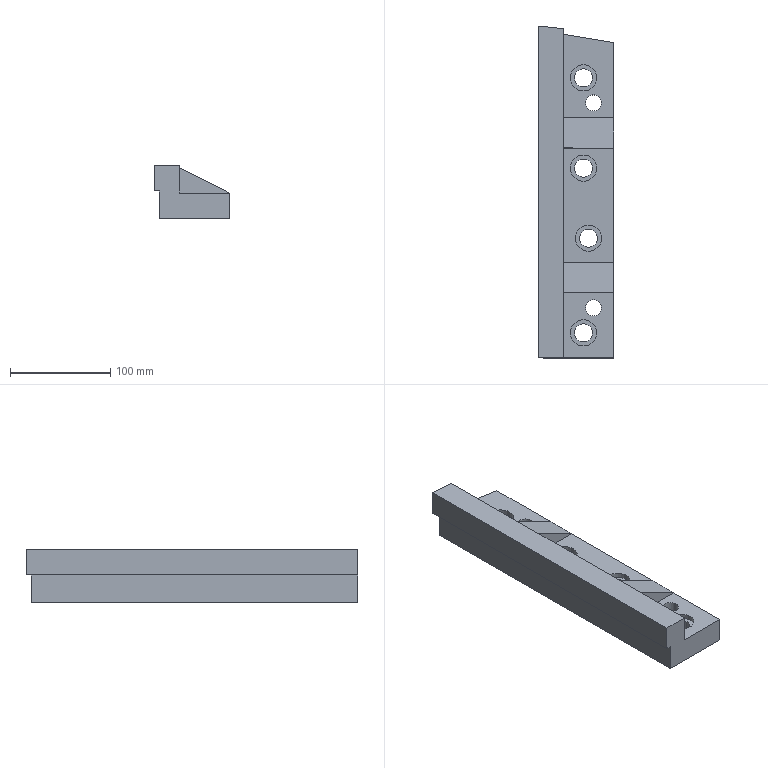Part | NX | features solid 2 | 1 solid | 33 faces | box 75 x 331.183 x 52 mm | volume 776457 mm3 | plane 21 | cylinder 10 | spline 2 | commonest cylinder face diameters 18 x4 26 x4 16 x2
STEP:
#1=CARTESIAN_POINT('',(-267.,-375.538,-30.));
#2=VERTEX_POINT('',#1);
#3=CARTESIAN_POINT('',(-280.,-375.538,-30.));
#4=DIRECTION('',(0.,0.,-1.));
#5=DIRECTION('',(1.,0.,0.));
#6=AXIS2_PLACEMENT_3D('',#3,#4,#5);
#7=CIRCLE('',#6,13.);
#8=EDGE_CURVE('',#2,#2,#7,.T.);
#9=ORIENTED_EDGE('',*,*,#8,.T.);
#10=EDGE_LOOP('',(#9));
#11=FACE_BOUND('',#10,.T.);
#12=CARTESIAN_POINT('',(-262.,-445.538,-30.));
#13=VERTEX_POINT('',#12);
#14=CARTESIAN_POINT('',(-275.,-445.538,-30.));
#15=DIRECTION('',(0.,0.,-1.));
#16=DIRECTION('',(1.,0.,0.));
#17=AXIS2_PLACEMENT_3D('',#14,#15,#16);
#18=CIRCLE('',#17,13.);
#19=EDGE_CURVE('',#13,#13,#18,.T.);
#20=ORIENTED_EDGE('',*,*,#19,.T.);
#21=EDGE_LOOP('',(#20));
#22=FACE_BOUND('',#21,.T.);
#23=CARTESIAN_POINT('',(-250.,-470.,-30.));
#24=VERTEX_POINT('',#23);
#25=CARTESIAN_POINT('',(-250.,-355.538,-30.));
#26=VERTEX_POINT('',#25);
#27=CARTESIAN_POINT('',(-250.,-560.,-30.));
#28=DIRECTION('',(0.,1.,0.));
#29=VECTOR('',#28,1000.);
#30=LINE('',#27,#29);
#31=EDGE_CURVE('',#24,#26,#30,.T.);
#32=ORIENTED_EDGE('',*,*,#31,.T.);
#33=CARTESIAN_POINT('',(-300.,-355.538,-30.));
#34=VERTEX_POINT('',#33);
#35=CARTESIAN_POINT('',(-300.,-355.538,-30.));
#36=DIRECTION('',(1.,0.,0.));
#37=VECTOR('',#36,1000.);
#38=LINE('',#35,#37);
#39=EDGE_CURVE('',#34,#26,#38,.T.);
#40=ORIENTED_EDGE('',*,*,#39,.F.);
#41=CARTESIAN_POINT('',(-300.,-470.,-30.));
#42=VERTEX_POINT('',#41);
#43=CARTESIAN_POINT('',(-300.,-560.,-30.));
#44=DIRECTION('',(0.,1.,0.));
#45=VECTOR('',#44,1000.);
#46=LINE('',#43,#45);
#47=EDGE_CURVE('',#42,#34,#46,.T.);
#48=ORIENTED_EDGE('',*,*,#47,.F.);
#49=CARTESIAN_POINT('',(-300.,-470.,-30.));
#50=DIRECTION('',(1.,0.,0.));
#51=VECTOR('',#50,1000.);
#52=LINE('',#49,#51);
#53=EDGE_CURVE('',#42,#24,#52,.T.);
#54=ORIENTED_EDGE('',*,*,#53,.T.);
#55=EDGE_LOOP('',(#32,#40,#48,#54));
#56=FACE_BOUND('',#55,.T.);
#57=CARTESIAN_POINT('',(-272.356,-257.29,-30.));
#58=DIRECTION('',(0.,0.,-1.));
#59=DIRECTION('',(-1.,0.,0.));
#60=AXIS2_PLACEMENT_3D('',#57,#58,#59);
#61=PLANE('',#60);
#62=ADVANCED_FACE('',(#11,#22,#56),#61,.F.);
#63=CARTESIAN_POINT('',(-267.,-285.538,-30.));
#64=VERTEX_POINT('',#63);
#65=CARTESIAN_POINT('',(-280.,-285.538,-30.));
#66=DIRECTION('',(0.,0.,-1.));
#67=DIRECTION('',(1.,0.,0.));
#68=AXIS2_PLACEMENT_3D('',#65,#66,#67);
#69=CIRCLE('',#68,13.);
#70=EDGE_CURVE('',#64,#64,#69,.T.);
#71=ORIENTED_EDGE('',*,*,#70,.T.);
#72=EDGE_LOOP('',(#71));
#73=FACE_BOUND('',#72,.T.);
#74=CARTESIAN_POINT('',(-262.,-310.538,-30.));
#75=VERTEX_POINT('',#74);
#76=CARTESIAN_POINT('',(-270.,-310.538,-30.));
#77=DIRECTION('',(0.,0.,-1.));
#78=DIRECTION('',(1.,0.,0.));
#79=AXIS2_PLACEMENT_3D('',#76,#77,#78);
#80=CIRCLE('',#79,8.);
#81=EDGE_CURVE('',#75,#75,#80,.T.);
#82=ORIENTED_EDGE('',*,*,#81,.T.);
#83=EDGE_LOOP('',(#82));
#84=FACE_BOUND('',#83,.T.);
#85=CARTESIAN_POINT('',(-300.,-325.538,-30.));
#86=VERTEX_POINT('',#85);
#87=CARTESIAN_POINT('',(-300.,-241.994,-30.));
#88=VERTEX_POINT('',#87);
#89=CARTESIAN_POINT('',(-300.,-560.,-30.));
#90=DIRECTION('',(0.,1.,0.));
#91=VECTOR('',#90,1000.);
#92=LINE('',#89,#91);
#93=EDGE_CURVE('',#86,#88,#92,.T.);
#94=ORIENTED_EDGE('',*,*,#93,.F.);
#95=CARTESIAN_POINT('',(-250.,-325.538,-30.));
#96=VERTEX_POINT('',#95);
#97=CARTESIAN_POINT('',(-300.,-325.538,-30.));
#98=DIRECTION('',(1.,0.,0.));
#99=VECTOR('',#98,1000.);
#100=LINE('',#97,#99);
#101=EDGE_CURVE('',#86,#96,#100,.T.);
#102=ORIENTED_EDGE('',*,*,#101,.T.);
#103=CARTESIAN_POINT('',(-250.,-250.331,-30.));
#104=VERTEX_POINT('',#103);
#105=CARTESIAN_POINT('',(-250.,-560.,-30.));
#106=DIRECTION('',(0.,1.,0.));
#107=VECTOR('',#106,1000.);
#108=LINE('',#105,#107);
#109=EDGE_CURVE('',#96,#104,#108,.T.);
#110=ORIENTED_EDGE('',*,*,#109,.T.);
#111=CARTESIAN_POINT('',(-250.,-250.331,-30.));
#112=CARTESIAN_POINT('',(-266.667,-247.552,-30.));
#113=CARTESIAN_POINT('',(-283.328,-244.74,-30.));
#114=CARTESIAN_POINT('',(-300.,-241.994,-30.));
#115=B_SPLINE_CURVE_WITH_KNOTS('',3,(#111,#112,#113,#114),.UNSPECIFIED.,.F.,.F.,(4,4),(0.3212,0.3719),.UNSPECIFIED.);
#116=EDGE_CURVE('',#104,#88,#115,.T.);
#117=ORIENTED_EDGE('',*,*,#116,.T.);
#118=EDGE_LOOP('',(#94,#102,#110,#117));
#119=FACE_BOUND('',#118,.T.);
#120=CARTESIAN_POINT('',(-272.356,-257.29,-30.));
#121=DIRECTION('',(0.,0.,-1.));
#122=DIRECTION('',(-1.,0.,0.));
#123=AXIS2_PLACEMENT_3D('',#120,#121,#122);
#124=PLANE('',#123);
#125=ADVANCED_FACE('',(#73,#84,#119),#124,.F.);
#126=CARTESIAN_POINT('',(-250.,-565.,-30.));
#127=VERTEX_POINT('',#126);
#128=CARTESIAN_POINT('',(-250.,-500.,-30.));
#129=VERTEX_POINT('',#128);
#130=CARTESIAN_POINT('',(-250.,-560.,-30.));
#131=DIRECTION('',(0.,1.,0.));
#132=VECTOR('',#131,1000.);
#133=LINE('',#130,#132);
#134=EDGE_CURVE('',#127,#129,#133,.T.);
#135=ORIENTED_EDGE('',*,*,#134,.T.);
#136=CARTESIAN_POINT('',(-300.,-500.,-30.));
#137=VERTEX_POINT('',#136);
#138=CARTESIAN_POINT('',(-300.,-500.,-30.));
#139=DIRECTION('',(1.,0.,0.));
#140=VECTOR('',#139,1000.);
#141=LINE('',#138,#140);
#142=EDGE_CURVE('',#137,#129,#141,.T.);
#143=ORIENTED_EDGE('',*,*,#142,.F.);
#144=CARTESIAN_POINT('',(-300.,-565.,-30.));
#145=VERTEX_POINT('',#144);
#146=CARTESIAN_POINT('',(-300.,-560.,-30.));
#147=DIRECTION('',(0.,1.,0.));
#148=VECTOR('',#147,1000.);
#149=LINE('',#146,#148);
#150=EDGE_CURVE('',#145,#137,#149,.T.);
#151=ORIENTED_EDGE('',*,*,#150,.F.);
#152=CARTESIAN_POINT('',(-245.,-565.,-30.));
#153=DIRECTION('',(-1.,0.,0.));
#154=VECTOR('',#153,1000.);
#155=LINE('',#152,#154);
#156=EDGE_CURVE('',#127,#145,#155,.T.);
#157=ORIENTED_EDGE('',*,*,#156,.F.);
#158=EDGE_LOOP('',(#135,#143,#151,#157));
#159=FACE_BOUND('',#158,.T.);
#160=CARTESIAN_POINT('',(-262.,-515.,-30.));
#161=VERTEX_POINT('',#160);
#162=CARTESIAN_POINT('',(-270.,-515.,-30.));
#163=DIRECTION('',(0.,0.,1.));
#164=DIRECTION('',(1.,0.,0.));
#165=AXIS2_PLACEMENT_3D('',#162,#163,#164);
#166=CIRCLE('',#165,8.);
#167=EDGE_CURVE('',#161,#161,#166,.T.);
#168=ORIENTED_EDGE('',*,*,#167,.F.);
#169=EDGE_LOOP('',(#168));
#170=FACE_BOUND('',#169,.T.);
#171=CARTESIAN_POINT('',(-267.,-540.,-30.));
#172=VERTEX_POINT('',#171);
#173=CARTESIAN_POINT('',(-280.,-540.,-30.));
#174=DIRECTION('',(0.,0.,1.));
#175=DIRECTION('',(1.,0.,0.));
#176=AXIS2_PLACEMENT_3D('',#173,#174,#175);
#177=CIRCLE('',#176,13.);
#178=EDGE_CURVE('',#172,#172,#177,.T.);
#179=ORIENTED_EDGE('',*,*,#178,.F.);
#180=EDGE_LOOP('',(#179));
#181=FACE_BOUND('',#180,.T.);
#182=CARTESIAN_POINT('',(-272.356,-257.29,-30.));
#183=DIRECTION('',(0.,0.,-1.));
#184=DIRECTION('',(-1.,0.,0.));
#185=AXIS2_PLACEMENT_3D('',#182,#183,#184);
#186=PLANE('',#185);
#187=ADVANCED_FACE('',(#159,#170,#181),#186,.F.);
#188=CARTESIAN_POINT('',(-289.,-540.,-55.));
#189=VERTEX_POINT('',#188);
#190=CARTESIAN_POINT('',(-280.,-540.,-55.));
#191=DIRECTION('',(0.,0.,-1.));
#192=DIRECTION('',(-1.,0.,0.));
#193=AXIS2_PLACEMENT_3D('',#190,#191,#192);
#194=CIRCLE('',#193,9.);
#195=EDGE_CURVE('',#189,#189,#194,.T.);
#196=ORIENTED_EDGE('',*,*,#195,.T.);
#197=EDGE_LOOP('',(#196));
#198=FACE_BOUND('',#197,.T.);
#199=CARTESIAN_POINT('',(-271.,-540.,-35.));
#200=VERTEX_POINT('',#199);
#201=CARTESIAN_POINT('',(-280.,-540.,-35.));
#202=DIRECTION('',(0.,0.,1.));
#203=DIRECTION('',(1.,0.,0.));
#204=AXIS2_PLACEMENT_3D('',#201,#202,#203);
#205=CIRCLE('',#204,9.);
#206=EDGE_CURVE('',#200,#200,#205,.F.);
#207=ORIENTED_EDGE('',*,*,#206,.F.);
#208=EDGE_LOOP('',(#207));
#209=FACE_BOUND('',#208,.T.);
#210=CARTESIAN_POINT('',(-280.,-540.,-60.));
#211=DIRECTION('',(0.,0.,1.));
#212=DIRECTION('',(1.,0.,0.));
#213=AXIS2_PLACEMENT_3D('',#210,#211,#212);
#214=CYLINDRICAL_SURFACE('',#213,9.);
#215=ADVANCED_FACE('',(#198,#209),#214,.F.);
#216=ORIENTED_EDGE('',*,*,#195,.F.);
#217=EDGE_LOOP('',(#216));
#218=FACE_BOUND('',#217,.T.);
#219=CARTESIAN_POINT('',(-278.,-515.,-55.));
#220=VERTEX_POINT('',#219);
#221=CARTESIAN_POINT('',(-270.,-515.,-55.));
#222=DIRECTION('',(0.,0.,-1.));
#223=DIRECTION('',(-1.,0.,0.));
#224=AXIS2_PLACEMENT_3D('',#221,#222,#223);
#225=CIRCLE('',#224,8.);
#226=EDGE_CURVE('',#220,#220,#225,.T.);
#227=ORIENTED_EDGE('',*,*,#226,.F.);
#228=EDGE_LOOP('',(#227));
#229=FACE_BOUND('',#228,.T.);
#230=CARTESIAN_POINT('',(-289.,-375.538,-55.));
#231=VERTEX_POINT('',#230);
#232=CARTESIAN_POINT('',(-280.,-375.538,-55.));
#233=DIRECTION('',(0.,0.,-1.));
#234=DIRECTION('',(-1.,0.,0.));
#235=AXIS2_PLACEMENT_3D('',#232,#233,#234);
#236=CIRCLE('',#235,9.);
#237=EDGE_CURVE('',#231,#231,#236,.F.);
#238=ORIENTED_EDGE('',*,*,#237,.T.);
#239=EDGE_LOOP('',(#238));
#240=FACE_BOUND('',#239,.T.);
#241=CARTESIAN_POINT('',(-289.,-285.538,-55.));
#242=VERTEX_POINT('',#241);
#243=CARTESIAN_POINT('',(-280.,-285.538,-55.));
#244=DIRECTION('',(0.,0.,-1.));
#245=DIRECTION('',(-1.,0.,0.));
#246=AXIS2_PLACEMENT_3D('',#243,#244,#245);
#247=CIRCLE('',#246,9.);
#248=EDGE_CURVE('',#242,#242,#247,.F.);
#249=ORIENTED_EDGE('',*,*,#248,.T.);
#250=EDGE_LOOP('',(#249));
#251=FACE_BOUND('',#250,.T.);
#252=CARTESIAN_POINT('',(-250.,-250.331,-55.));
#253=VERTEX_POINT('',#252);
#254=CARTESIAN_POINT('',(-320.,-238.927,-55.));
#255=VERTEX_POINT('',#254);
#256=CARTESIAN_POINT('',(-250.,-250.331,-55.));
#257=CARTESIAN_POINT('',(-261.66,-248.387,-55.));
#258=CARTESIAN_POINT('',(-284.979,-244.502,-55.));
#259=CARTESIAN_POINT('',(-308.296,-240.6,-55.));
#260=CARTESIAN_POINT('',(-320.,-238.927,-55.));
#261=B_SPLINE_CURVE_WITH_KNOTS('',3,(#256,#257,#258,#259,#260),.UNSPECIFIED.,.F.,.F.,(4,1,4),(0.,0.03546,0.07092),.UNSPECIFIED.);
#262=EDGE_CURVE('',#253,#255,#261,.T.);
#263=ORIENTED_EDGE('',*,*,#262,.F.);
#264=CARTESIAN_POINT('',(-250.,-565.,-55.));
#265=VERTEX_POINT('',#264);
#266=CARTESIAN_POINT('',(-250.,-560.,-55.));
#267=DIRECTION('',(0.,1.,0.));
#268=VECTOR('',#267,1000.);
#269=LINE('',#266,#268);
#270=EDGE_CURVE('',#265,#253,#269,.T.);
#271=ORIENTED_EDGE('',*,*,#270,.F.);
#272=CARTESIAN_POINT('',(-320.,-565.,-55.));
#273=VERTEX_POINT('',#272);
#274=CARTESIAN_POINT('',(-245.,-565.,-55.));
#275=DIRECTION('',(-1.,0.,0.));
#276=VECTOR('',#275,1000.);
#277=LINE('',#274,#276);
#278=EDGE_CURVE('',#265,#273,#277,.T.);
#279=ORIENTED_EDGE('',*,*,#278,.T.);
#280=CARTESIAN_POINT('',(-320.,-257.29,-55.));
#281=DIRECTION('',(0.,1.,0.));
#282=VECTOR('',#281,1000.);
#283=LINE('',#280,#282);
#284=EDGE_CURVE('',#273,#255,#283,.T.);
#285=ORIENTED_EDGE('',*,*,#284,.T.);
#286=EDGE_LOOP('',(#263,#271,#279,#285));
#287=FACE_BOUND('',#286,.T.);
#288=CARTESIAN_POINT('',(-278.,-310.538,-55.));
#289=VERTEX_POINT('',#288);
#290=CARTESIAN_POINT('',(-270.,-310.538,-55.));
#291=DIRECTION('',(0.,0.,-1.));
#292=DIRECTION('',(-1.,0.,0.));
#293=AXIS2_PLACEMENT_3D('',#290,#291,#292);
#294=CIRCLE('',#293,8.);
#295=EDGE_CURVE('',#289,#289,#294,.F.);
#296=ORIENTED_EDGE('',*,*,#295,.T.);
#297=EDGE_LOOP('',(#296));
#298=FACE_BOUND('',#297,.T.);
#299=CARTESIAN_POINT('',(-284.,-445.538,-55.));
#300=VERTEX_POINT('',#299);
#301=CARTESIAN_POINT('',(-275.,-445.538,-55.));
#302=DIRECTION('',(0.,0.,-1.));
#303=DIRECTION('',(-1.,0.,0.));
#304=AXIS2_PLACEMENT_3D('',#301,#302,#303);
#305=CIRCLE('',#304,9.);
#306=EDGE_CURVE('',#300,#300,#305,.F.);
#307=ORIENTED_EDGE('',*,*,#306,.T.);
#308=EDGE_LOOP('',(#307));
#309=FACE_BOUND('',#308,.T.);
#310=CARTESIAN_POINT('',(-272.356,-257.29,-55.));
#311=DIRECTION('',(0.,0.,-1.));
#312=DIRECTION('',(-1.,0.,0.));
#313=AXIS2_PLACEMENT_3D('',#310,#311,#312);
#314=PLANE('',#313);
#315=ADVANCED_FACE('',(#218,#229,#240,#251,#287,#298,#309),#314,.T.);
#316=CARTESIAN_POINT('',(-320.,-565.,-28.));
#317=VERTEX_POINT('',#316);
#318=CARTESIAN_POINT('',(-320.,-565.,-53.));
#319=DIRECTION('',(0.,0.,1.));
#320=VECTOR('',#319,1000.);
#321=LINE('',#318,#320);
#322=EDGE_CURVE('',#273,#317,#321,.T.);
#323=ORIENTED_EDGE('',*,*,#322,.F.);
#324=ORIENTED_EDGE('',*,*,#278,.F.);
#325=CARTESIAN_POINT('',(-250.,-565.,-53.));
#326=DIRECTION('',(0.,0.,1.));
#327=VECTOR('',#326,1000.);
#328=LINE('',#325,#327);
#329=EDGE_CURVE('',#265,#127,#328,.T.);
#330=ORIENTED_EDGE('',*,*,#329,.T.);
#331=ORIENTED_EDGE('',*,*,#156,.T.);
#332=CARTESIAN_POINT('',(-300.,-565.,-3.));
#333=VERTEX_POINT('',#332);
#334=CARTESIAN_POINT('',(-300.,-565.,-53.));
#335=DIRECTION('',(0.,0.,1.));
#336=VECTOR('',#335,1000.);
#337=LINE('',#334,#336);
#338=EDGE_CURVE('',#145,#333,#337,.T.);
#339=ORIENTED_EDGE('',*,*,#338,.T.);
#340=CARTESIAN_POINT('',(-325.,-565.,-3.));
#341=VERTEX_POINT('',#340);
#342=CARTESIAN_POINT('',(-245.,-565.,-3.));
#343=DIRECTION('',(-1.,0.,0.));
#344=VECTOR('',#343,1000.);
#345=LINE('',#342,#344);
#346=EDGE_CURVE('',#333,#341,#345,.T.);
#347=ORIENTED_EDGE('',*,*,#346,.T.);
#348=CARTESIAN_POINT('',(-325.,-565.,-28.));
#349=VERTEX_POINT('',#348);
#350=CARTESIAN_POINT('',(-325.,-565.,-53.));
#351=DIRECTION('',(0.,0.,1.));
#352=VECTOR('',#351,1000.);
#353=LINE('',#350,#352);
#354=EDGE_CURVE('',#349,#341,#353,.T.);
#355=ORIENTED_EDGE('',*,*,#354,.F.);
#356=CARTESIAN_POINT('',(-245.,-565.,-28.));
#357=DIRECTION('',(-1.,0.,0.));
#358=VECTOR('',#357,1000.);
#359=LINE('',#356,#358);
#360=EDGE_CURVE('',#317,#349,#359,.T.);
#361=ORIENTED_EDGE('',*,*,#360,.F.);
#362=EDGE_LOOP('',(#323,#324,#330,#331,#339,#347,#355,#361));
#363=FACE_BOUND('',#362,.T.);
#364=CARTESIAN_POINT('',(-245.,-565.,-53.));
#365=DIRECTION('',(0.,1.,0.));
#366=DIRECTION('',(0.,0.,1.));
#367=AXIS2_PLACEMENT_3D('',#364,#365,#366);
#368=PLANE('',#367);
#369=ADVANCED_FACE('',(#363),#368,.F.);
#370=CARTESIAN_POINT('',(-325.,-233.817,-3.));
#371=VERTEX_POINT('',#370);
#372=CARTESIAN_POINT('',(-325.,-560.,-3.));
#373=DIRECTION('',(0.,1.,0.));
#374=VECTOR('',#373,1000.);
#375=LINE('',#372,#374);
#376=EDGE_CURVE('',#341,#371,#375,.T.);
#377=ORIENTED_EDGE('',*,*,#376,.T.);
#378=CARTESIAN_POINT('',(-325.,-233.817,-28.));
#379=VERTEX_POINT('',#378);
#380=CARTESIAN_POINT('',(-325.,-233.817,-100.));
#381=DIRECTION('',(0.,0.,1.));
#382=VECTOR('',#381,1000.);
#383=LINE('',#380,#382);
#384=EDGE_CURVE('',#371,#379,#383,.F.);
#385=ORIENTED_EDGE('',*,*,#384,.T.);
#386=CARTESIAN_POINT('',(-325.,-560.,-28.));
#387=DIRECTION('',(0.,1.,0.));
#388=VECTOR('',#387,1000.);
#389=LINE('',#386,#388);
#390=EDGE_CURVE('',#349,#379,#389,.T.);
#391=ORIENTED_EDGE('',*,*,#390,.F.);
#392=ORIENTED_EDGE('',*,*,#354,.T.);
#393=EDGE_LOOP('',(#377,#385,#391,#392));
#394=FACE_BOUND('',#393,.T.);
#395=CARTESIAN_POINT('',(-325.,-560.,-53.));
#396=DIRECTION('',(1.,0.,0.));
#397=DIRECTION('',(0.,0.,-1.));
#398=AXIS2_PLACEMENT_3D('',#395,#396,#397);
#399=PLANE('',#398);
#400=ADVANCED_FACE('',(#394),#399,.F.);
#401=CARTESIAN_POINT('',(-250.,-250.331,-42.5));
#402=DIRECTION('',(0.,0.,-1.));
#403=VECTOR('',#402,1000.);
#404=LINE('',#401,#403);
#405=EDGE_CURVE('',#104,#253,#404,.T.);
#406=ORIENTED_EDGE('',*,*,#405,.F.);
#407=ORIENTED_EDGE('',*,*,#109,.F.);
#408=CARTESIAN_POINT('',(-250.,-355.538,-30.));
#409=DIRECTION('',(0.,1.,0.));
#410=VECTOR('',#409,1000.);
#411=LINE('',#408,#410);
#412=EDGE_CURVE('',#26,#96,#411,.T.);
#413=ORIENTED_EDGE('',*,*,#412,.F.);
#414=ORIENTED_EDGE('',*,*,#31,.F.);
#415=CARTESIAN_POINT('',(-250.,-470.,-30.));
#416=DIRECTION('',(0.,-1.,0.));
#417=VECTOR('',#416,1000.);
#418=LINE('',#415,#417);
#419=EDGE_CURVE('',#24,#129,#418,.T.);
#420=ORIENTED_EDGE('',*,*,#419,.T.);
#421=ORIENTED_EDGE('',*,*,#134,.F.);
#422=ORIENTED_EDGE('',*,*,#329,.F.);
#423=ORIENTED_EDGE('',*,*,#270,.T.);
#424=EDGE_LOOP('',(#406,#407,#413,#414,#420,#421,#422,#423));
#425=FACE_BOUND('',#424,.T.);
#426=CARTESIAN_POINT('',(-250.,-560.,-53.));
#427=DIRECTION('',(1.,0.,0.));
#428=DIRECTION('',(0.,0.,-1.));
#429=AXIS2_PLACEMENT_3D('',#426,#427,#428);
#430=PLANE('',#429);
#431=ADVANCED_FACE('',(#425),#430,.T.);
#432=CARTESIAN_POINT('',(-300.,-236.451,-3.));
#433=VERTEX_POINT('',#432);
#434=CARTESIAN_POINT('',(-300.,-236.451,-28.));
#435=VERTEX_POINT('',#434);
#436=CARTESIAN_POINT('',(-300.,-236.451,-100.));
#437=DIRECTION('',(0.,0.,1.));
#438=VECTOR('',#437,1000.);
#439=LINE('',#436,#438);
#440=EDGE_CURVE('',#433,#435,#439,.F.);
#441=ORIENTED_EDGE('',*,*,#440,.F.);
#442=CARTESIAN_POINT('',(-300.,-560.,-3.));
#443=DIRECTION('',(0.,1.,0.));
#444=VECTOR('',#443,1000.);
#445=LINE('',#442,#444);
#446=EDGE_CURVE('',#333,#433,#445,.T.);
#447=ORIENTED_EDGE('',*,*,#446,.F.);
#448=ORIENTED_EDGE('',*,*,#338,.F.);
#449=ORIENTED_EDGE('',*,*,#150,.T.);
#450=CARTESIAN_POINT('',(-300.,-500.,-5.));
#451=VERTEX_POINT('',#450);
#452=CARTESIAN_POINT('',(-300.,-500.,-30.));
#453=DIRECTION('',(0.,0.,1.));
#454=VECTOR('',#453,1000.);
#455=LINE('',#452,#454);
#456=EDGE_CURVE('',#137,#451,#455,.T.);
#457=ORIENTED_EDGE('',*,*,#456,.T.);
#458=CARTESIAN_POINT('',(-300.,-470.,-5.));
#459=VERTEX_POINT('',#458);
#460=CARTESIAN_POINT('',(-300.,-470.,-5.));
#461=DIRECTION('',(0.,1.,0.));
#462=VECTOR('',#461,1000.);
#463=LINE('',#460,#462);
#464=EDGE_CURVE('',#459,#451,#463,.F.);
#465=ORIENTED_EDGE('',*,*,#464,.F.);
#466=CARTESIAN_POINT('',(-300.,-470.,-30.));
#467=DIRECTION('',(0.,0.,1.));
#468=VECTOR('',#467,1000.);
#469=LINE('',#466,#468);
#470=EDGE_CURVE('',#42,#459,#469,.T.);
#471=ORIENTED_EDGE('',*,*,#470,.F.);
#472=ORIENTED_EDGE('',*,*,#47,.T.);
#473=CARTESIAN_POINT('',(-300.,-355.538,-5.));
#474=VERTEX_POINT('',#473);
#475=CARTESIAN_POINT('',(-300.,-355.538,-30.));
#476=DIRECTION('',(0.,0.,1.));
#477=VECTOR('',#476,1000.);
#478=LINE('',#475,#477);
#479=EDGE_CURVE('',#34,#474,#478,.T.);
#480=ORIENTED_EDGE('',*,*,#479,.T.);
#481=CARTESIAN_POINT('',(-300.,-325.538,-5.));
#482=VERTEX_POINT('',#481);
#483=CARTESIAN_POINT('',(-300.,-355.538,-5.));
#484=DIRECTION('',(0.,-1.,0.));
#485=VECTOR('',#484,1000.);
#486=LINE('',#483,#485);
#487=EDGE_CURVE('',#474,#482,#486,.F.);
#488=ORIENTED_EDGE('',*,*,#487,.T.);
#489=CARTESIAN_POINT('',(-300.,-325.538,-30.));
#490=DIRECTION('',(0.,0.,1.));
#491=VECTOR('',#490,1000.);
#492=LINE('',#489,#491);
#493=EDGE_CURVE('',#86,#482,#492,.T.);
#494=ORIENTED_EDGE('',*,*,#493,.F.);
#495=ORIENTED_EDGE('',*,*,#93,.T.);
#496=CARTESIAN_POINT('',(-300.,-241.994,-28.));
#497=VERTEX_POINT('',#496);
#498=CARTESIAN_POINT('',(-300.,-241.994,-29.));
#499=DIRECTION('',(0.,0.,-1.));
#500=VECTOR('',#499,1000.);
#501=LINE('',#498,#500);
#502=EDGE_CURVE('',#497,#88,#501,.T.);
#503=ORIENTED_EDGE('',*,*,#502,.F.);
#504=CARTESIAN_POINT('',(-300.,-560.,-28.));
#505=DIRECTION('',(0.,-1.,0.));
#506=VECTOR('',#505,1000.);
#507=LINE('',#504,#506);
#508=EDGE_CURVE('',#435,#497,#507,.T.);
#509=ORIENTED_EDGE('',*,*,#508,.F.);
#510=EDGE_LOOP('',(#441,#447,#448,#449,#457,#465,#471,#472,#480,#488,#494,#495,#503,#509));
#511=FACE_BOUND('',#510,.T.);
#512=CARTESIAN_POINT('',(-300.,-560.,-53.));
#513=DIRECTION('',(1.,0.,0.));
#514=DIRECTION('',(0.,0.,-1.));
#515=AXIS2_PLACEMENT_3D('',#512,#513,#514);
#516=PLANE('',#515);
#517=ADVANCED_FACE('',(#511),#516,.T.);
#518=ORIENTED_EDGE('',*,*,#446,.T.);
#519=CARTESIAN_POINT('',(-467.332,-211.778,-3.));
#520=CARTESIAN_POINT('',(-453.683,-214.296,-3.));
#521=CARTESIAN_POINT('',(-426.385,-219.33,-3.));
#522=CARTESIAN_POINT('',(-385.36,-226.473,-3.));
#523=CARTESIAN_POINT('',(-344.075,-231.948,-3.));
#524=CARTESIAN_POINT('',(-302.639,-236.064,-3.));
#525=CARTESIAN_POINT('',(-261.264,-240.795,-3.));
#526=CARTESIAN_POINT('',(-220.344,-248.886,-3.));
#527=CARTESIAN_POINT('',(-187.701,-261.197,-3.));
#528=CARTESIAN_POINT('',(-163.887,-275.581,-3.));
#529=CARTESIAN_POINT('',(-147.555,-288.567,-3.));
#530=CARTESIAN_POINT('',(-132.971,-303.448,-3.));
#531=CARTESIAN_POINT('',(-115.628,-325.186,-3.));
#532=CARTESIAN_POINT('',(-97.34,-354.727,-3.));
#533=CARTESIAN_POINT('',(-77.186,-391.16,-3.));
#534=CARTESIAN_POINT('',(-55.898,-426.958,-3.));
#535=CARTESIAN_POINT('',(-32.602,-461.482,-3.));
#536=CARTESIAN_POINT('',(-11.577,-489.134,-3.));
#537=CARTESIAN_POINT('',(7.388,-509.445,-3.));
#538=CARTESIAN_POINT('',(23.204,-523.049,-3.));
#539=CARTESIAN_POINT('',(37.741,-532.559,-3.));
#540=CARTESIAN_POINT('',(49.762,-539.511,-3.));
#541=CARTESIAN_POINT('',(58.522,-544.87,-3.));
#542=CARTESIAN_POINT('',(66.969,-550.477,-3.));
#543=CARTESIAN_POINT('',(72.545,-554.13,-3.));
#544=CARTESIAN_POINT('',(75.334,-555.957,-3.));
#545=B_SPLINE_CURVE_WITH_KNOTS('',3,(#519,#520,#521,#522,#523,#524,#525,#526,#527,#528,#529,#530,#531,#532,#533,#534,#535,#536,#537,#538,#539,#540,#541,#542,#543,#544),.UNSPECIFIED.,.F.,.F.,(4,1,1,1,1,1,1,1,1,1,1,1,1,1,1,1,1,1,1,1,1,1,1,4),(0.392,0.4289,0.4658,0.5026,0.5395,0.5764,0.6133,0.6502,0.6687,0.6871,0.7056,0.724,0.7609,0.7978,0.8347,0.8716,0.9085,0.9269,0.9454,0.9638,0.9731,0.9823,0.9911,1.),.UNSPECIFIED.);
#546=EDGE_CURVE('',#433,#371,#545,.F.);
#547=ORIENTED_EDGE('',*,*,#546,.T.);
#548=ORIENTED_EDGE('',*,*,#376,.F.);
#549=ORIENTED_EDGE('',*,*,#346,.F.);
#550=EDGE_LOOP('',(#518,#547,#548,#549));
#551=FACE_BOUND('',#550,.T.);
#552=CARTESIAN_POINT('',(-312.488,-250.142,-3.));
#553=DIRECTION('',(0.,0.,-1.));
#554=DIRECTION('',(-1.,0.,0.));
#555=AXIS2_PLACEMENT_3D('',#552,#553,#554);
#556=PLANE('',#555);
#557=ADVANCED_FACE('',(#551),#556,.F.);
#558=CARTESIAN_POINT('',(-467.332,-211.778,-28.));
#559=CARTESIAN_POINT('',(-453.683,-214.296,-28.));
#560=CARTESIAN_POINT('',(-426.385,-219.33,-28.));
#561=CARTESIAN_POINT('',(-385.36,-226.473,-28.));
#562=CARTESIAN_POINT('',(-344.075,-231.948,-28.));
#563=CARTESIAN_POINT('',(-302.639,-236.064,-28.));
#564=CARTESIAN_POINT('',(-261.264,-240.795,-28.));
#565=CARTESIAN_POINT('',(-220.344,-248.886,-28.));
#566=CARTESIAN_POINT('',(-187.701,-261.197,-28.));
#567=CARTESIAN_POINT('',(-163.887,-275.581,-28.));
#568=CARTESIAN_POINT('',(-147.555,-288.567,-28.));
#569=CARTESIAN_POINT('',(-132.971,-303.448,-28.));
#570=CARTESIAN_POINT('',(-115.628,-325.186,-28.));
#571=CARTESIAN_POINT('',(-97.34,-354.727,-28.));
#572=CARTESIAN_POINT('',(-77.186,-391.16,-28.));
#573=CARTESIAN_POINT('',(-55.898,-426.958,-28.));
#574=CARTESIAN_POINT('',(-32.602,-461.482,-28.));
#575=CARTESIAN_POINT('',(-11.577,-489.134,-28.));
#576=CARTESIAN_POINT('',(7.388,-509.445,-28.));
#577=CARTESIAN_POINT('',(23.204,-523.049,-28.));
#578=CARTESIAN_POINT('',(37.741,-532.559,-28.));
#579=CARTESIAN_POINT('',(49.762,-539.511,-28.));
#580=CARTESIAN_POINT('',(58.522,-544.87,-28.));
#581=CARTESIAN_POINT('',(66.969,-550.477,-28.));
#582=CARTESIAN_POINT('',(72.545,-554.13,-28.));
#583=CARTESIAN_POINT('',(75.334,-555.957,-28.));
#584=B_SPLINE_CURVE_WITH_KNOTS('',3,(#558,#559,#560,#561,#562,#563,#564,#565,#566,#567,#568,#569,#570,#571,#572,#573,#574,#575,#576,#577,#578,#579,#580,#581,#582,#583),.UNSPECIFIED.,.F.,.F.,(4,1,1,1,1,1,1,1,1,1,1,1,1,1,1,1,1,1,1,1,1,1,1,4),(0.392,0.4289,0.4658,0.5026,0.5395,0.5764,0.6133,0.6502,0.6687,0.6871,0.7056,0.724,0.7609,0.7978,0.8347,0.8716,0.9085,0.9269,0.9454,0.9638,0.9731,0.9823,0.9911,1.),.UNSPECIFIED.);
#585=EDGE_CURVE('',#435,#379,#584,.F.);
#586=ORIENTED_EDGE('',*,*,#585,.F.);
#587=ORIENTED_EDGE('',*,*,#508,.T.);
#588=CARTESIAN_POINT('',(-320.,-238.927,-28.));
#589=VERTEX_POINT('',#588);
#590=CARTESIAN_POINT('',(-300.,-241.994,-28.));
#591=CARTESIAN_POINT('',(-306.655,-240.898,-28.));
#592=CARTESIAN_POINT('',(-313.323,-239.882,-28.));
#593=CARTESIAN_POINT('',(-320.,-238.927,-28.));
#594=B_SPLINE_CURVE_WITH_KNOTS('',3,(#590,#591,#592,#593),.UNSPECIFIED.,.F.,.F.,(4,4),(0.103,0.1232),.UNSPECIFIED.);
#595=EDGE_CURVE('',#497,#589,#594,.T.);
#596=ORIENTED_EDGE('',*,*,#595,.T.);
#597=CARTESIAN_POINT('',(-320.,-560.,-28.));
#598=DIRECTION('',(0.,1.,0.));
#599=VECTOR('',#598,1000.);
#600=LINE('',#597,#599);
#601=EDGE_CURVE('',#317,#589,#600,.T.);
#602=ORIENTED_EDGE('',*,*,#601,.F.);
#603=ORIENTED_EDGE('',*,*,#360,.T.);
#604=ORIENTED_EDGE('',*,*,#390,.T.);
#605=EDGE_LOOP('',(#586,#587,#596,#602,#603,#604));
#606=FACE_BOUND('',#605,.T.);
#607=CARTESIAN_POINT('',(-300.,-560.,-28.));
#608=DIRECTION('',(0.,0.,-1.));
#609=DIRECTION('',(-1.,0.,0.));
#610=AXIS2_PLACEMENT_3D('',#607,#608,#609);
#611=PLANE('',#610);
#612=ADVANCED_FACE('',(#606),#611,.T.);
#613=CARTESIAN_POINT('',(-320.,-238.927,-41.5));
#614=DIRECTION('',(0.,0.,-1.));
#615=VECTOR('',#614,1000.);
#616=LINE('',#613,#615);
#617=EDGE_CURVE('',#255,#589,#616,.F.);
#618=ORIENTED_EDGE('',*,*,#617,.F.);
#619=ORIENTED_EDGE('',*,*,#284,.F.);
#620=ORIENTED_EDGE('',*,*,#322,.T.);
#621=ORIENTED_EDGE('',*,*,#601,.T.);
#622=EDGE_LOOP('',(#618,#619,#620,#621));
#623=FACE_BOUND('',#622,.T.);
#624=CARTESIAN_POINT('',(-320.,-560.,-28.));
#625=DIRECTION('',(-1.,0.,0.));
#626=DIRECTION('',(0.,0.,1.));
#627=AXIS2_PLACEMENT_3D('',#624,#625,#626);
#628=PLANE('',#627);
#629=ADVANCED_FACE('',(#623),#628,.T.);
#630=ORIENTED_EDGE('',*,*,#405,.T.);
#631=ORIENTED_EDGE('',*,*,#262,.T.);
#632=ORIENTED_EDGE('',*,*,#617,.T.);
#633=ORIENTED_EDGE('',*,*,#595,.F.);
#634=ORIENTED_EDGE('',*,*,#502,.T.);
#635=ORIENTED_EDGE('',*,*,#116,.F.);
#636=EDGE_LOOP('',(#630,#631,#632,#633,#634,#635));
#637=FACE_BOUND('',#636,.T.);
#638=CARTESIAN_POINT('',(-250.,-250.331,-28.));
#639=CARTESIAN_POINT('',(-250.,-250.331,-55.));
#640=CARTESIAN_POINT('',(-261.622,-248.393,-28.));
#641=CARTESIAN_POINT('',(-261.622,-248.393,-55.));
#642=CARTESIAN_POINT('',(-279.055,-245.51,-28.));
#643=CARTESIAN_POINT('',(-279.055,-245.51,-55.));
#644=CARTESIAN_POINT('',(-302.299,-241.568,-28.));
#645=CARTESIAN_POINT('',(-302.299,-241.568,-55.));
#646=CARTESIAN_POINT('',(-314.116,-239.768,-28.));
#647=CARTESIAN_POINT('',(-314.116,-239.768,-55.));
#648=CARTESIAN_POINT('',(-320.,-238.927,-28.));
#649=CARTESIAN_POINT('',(-320.,-238.927,-55.));
#650=B_SPLINE_SURFACE_WITH_KNOTS('',3,1,((#638,#639),(#640,#641),(#642,#643),(#644,#645),(#646,#647),(#648,#649)),.SURF_OF_LINEAR_EXTRUSION.,.F.,.F.,.F.,(4,1,1,4),(2,2),(-1.938,-0.5407,0.1581,0.8568),(0.,1.),.UNSPECIFIED.);
#651=ADVANCED_FACE('',(#637),#650,.F.);
#652=CARTESIAN_POINT('',(-289.,-285.538,-35.));
#653=VERTEX_POINT('',#652);
#654=CARTESIAN_POINT('',(-280.,-285.538,-35.));
#655=DIRECTION('',(0.,0.,-1.));
#656=DIRECTION('',(-1.,0.,0.));
#657=AXIS2_PLACEMENT_3D('',#654,#655,#656);
#658=CIRCLE('',#657,9.);
#659=EDGE_CURVE('',#653,#653,#658,.T.);
#660=ORIENTED_EDGE('',*,*,#659,.F.);
#661=EDGE_LOOP('',(#660));
#662=FACE_BOUND('',#661,.T.);
#663=ORIENTED_EDGE('',*,*,#248,.F.);
#664=EDGE_LOOP('',(#663));
#665=FACE_BOUND('',#664,.T.);
#666=CARTESIAN_POINT('',(-280.,-285.538,-60.));
#667=DIRECTION('',(0.,0.,1.));
#668=DIRECTION('',(1.,0.,0.));
#669=AXIS2_PLACEMENT_3D('',#666,#667,#668);
#670=CYLINDRICAL_SURFACE('',#669,9.);
#671=ADVANCED_FACE('',(#662,#665),#670,.F.);
#672=ORIENTED_EDGE('',*,*,#295,.F.);
#673=EDGE_LOOP('',(#672));
#674=FACE_BOUND('',#673,.T.);
#675=ORIENTED_EDGE('',*,*,#81,.F.);
#676=EDGE_LOOP('',(#675));
#677=FACE_BOUND('',#676,.T.);
#678=CARTESIAN_POINT('',(-270.,-310.538,-60.));
#679=DIRECTION('',(0.,0.,1.));
#680=DIRECTION('',(1.,0.,0.));
#681=AXIS2_PLACEMENT_3D('',#678,#679,#680);
#682=CYLINDRICAL_SURFACE('',#681,8.);
#683=ADVANCED_FACE('',(#674,#677),#682,.F.);
#684=CARTESIAN_POINT('',(-289.,-375.538,-35.));
#685=VERTEX_POINT('',#684);
#686=CARTESIAN_POINT('',(-280.,-375.538,-35.));
#687=DIRECTION('',(0.,0.,-1.));
#688=DIRECTION('',(-1.,0.,0.));
#689=AXIS2_PLACEMENT_3D('',#686,#687,#688);
#690=CIRCLE('',#689,9.);
#691=EDGE_CURVE('',#685,#685,#690,.T.);
#692=ORIENTED_EDGE('',*,*,#691,.F.);
#693=EDGE_LOOP('',(#692));
#694=FACE_BOUND('',#693,.T.);
#695=ORIENTED_EDGE('',*,*,#237,.F.);
#696=EDGE_LOOP('',(#695));
#697=FACE_BOUND('',#696,.T.);
#698=CARTESIAN_POINT('',(-280.,-375.538,-60.));
#699=DIRECTION('',(0.,0.,1.));
#700=DIRECTION('',(1.,0.,0.));
#701=AXIS2_PLACEMENT_3D('',#698,#699,#700);
#702=CYLINDRICAL_SURFACE('',#701,9.);
#703=ADVANCED_FACE('',(#694,#697),#702,.F.);
#704=CARTESIAN_POINT('',(-284.,-445.538,-35.));
#705=VERTEX_POINT('',#704);
#706=CARTESIAN_POINT('',(-275.,-445.538,-35.));
#707=DIRECTION('',(0.,0.,-1.));
#708=DIRECTION('',(-1.,0.,0.));
#709=AXIS2_PLACEMENT_3D('',#706,#707,#708);
#710=CIRCLE('',#709,9.);
#711=EDGE_CURVE('',#705,#705,#710,.T.);
#712=ORIENTED_EDGE('',*,*,#711,.F.);
#713=EDGE_LOOP('',(#712));
#714=FACE_BOUND('',#713,.T.);
#715=ORIENTED_EDGE('',*,*,#306,.F.);
#716=EDGE_LOOP('',(#715));
#717=FACE_BOUND('',#716,.T.);
#718=CARTESIAN_POINT('',(-275.,-445.538,-60.));
#719=DIRECTION('',(0.,0.,1.));
#720=DIRECTION('',(1.,0.,0.));
#721=AXIS2_PLACEMENT_3D('',#718,#719,#720);
#722=CYLINDRICAL_SURFACE('',#721,9.);
#723=ADVANCED_FACE('',(#714,#717),#722,.F.);
#724=ORIENTED_EDGE('',*,*,#226,.T.);
#725=EDGE_LOOP('',(#724));
#726=FACE_BOUND('',#725,.T.);
#727=ORIENTED_EDGE('',*,*,#167,.T.);
#728=EDGE_LOOP('',(#727));
#729=FACE_BOUND('',#728,.T.);
#730=CARTESIAN_POINT('',(-270.,-515.,-60.));
#731=DIRECTION('',(0.,0.,1.));
#732=DIRECTION('',(1.,0.,0.));
#733=AXIS2_PLACEMENT_3D('',#730,#731,#732);
#734=CYLINDRICAL_SURFACE('',#733,8.);
#735=ADVANCED_FACE('',(#726,#729),#734,.F.);
#736=CARTESIAN_POINT('',(-267.,-540.,-35.));
#737=VERTEX_POINT('',#736);
#738=CARTESIAN_POINT('',(-280.,-540.,-35.));
#739=DIRECTION('',(0.,0.,1.));
#740=DIRECTION('',(1.,0.,0.));
#741=AXIS2_PLACEMENT_3D('',#738,#739,#740);
#742=CIRCLE('',#741,13.);
#743=EDGE_CURVE('',#737,#737,#742,.T.);
#744=ORIENTED_EDGE('',*,*,#743,.T.);
#745=EDGE_LOOP('',(#744));
#746=FACE_BOUND('',#745,.T.);
#747=ORIENTED_EDGE('',*,*,#206,.T.);
#748=EDGE_LOOP('',(#747));
#749=FACE_BOUND('',#748,.T.);
#750=CARTESIAN_POINT('',(-280.,-540.,-35.));
#751=DIRECTION('',(0.,0.,1.));
#752=DIRECTION('',(1.,0.,0.));
#753=AXIS2_PLACEMENT_3D('',#750,#751,#752);
#754=PLANE('',#753);
#755=ADVANCED_FACE('',(#746,#749),#754,.T.);
#756=ORIENTED_EDGE('',*,*,#743,.F.);
#757=EDGE_LOOP('',(#756));
#758=FACE_BOUND('',#757,.T.);
#759=ORIENTED_EDGE('',*,*,#178,.T.);
#760=EDGE_LOOP('',(#759));
#761=FACE_BOUND('',#760,.T.);
#762=CARTESIAN_POINT('',(-280.,-540.,-35.));
#763=DIRECTION('',(0.,0.,1.));
#764=DIRECTION('',(1.,0.,0.));
#765=AXIS2_PLACEMENT_3D('',#762,#763,#764);
#766=CYLINDRICAL_SURFACE('',#765,13.);
#767=ADVANCED_FACE('',(#758,#761),#766,.F.);
#768=CARTESIAN_POINT('',(-262.,-445.538,-35.));
#769=VERTEX_POINT('',#768);
#770=CARTESIAN_POINT('',(-275.,-445.538,-35.));
#771=DIRECTION('',(0.,0.,-1.));
#772=DIRECTION('',(1.,0.,0.));
#773=AXIS2_PLACEMENT_3D('',#770,#771,#772);
#774=CIRCLE('',#773,13.);
#775=EDGE_CURVE('',#769,#769,#774,.T.);
#776=ORIENTED_EDGE('',*,*,#775,.T.);
#777=EDGE_LOOP('',(#776));
#778=FACE_BOUND('',#777,.T.);
#779=ORIENTED_EDGE('',*,*,#19,.F.);
#780=EDGE_LOOP('',(#779));
#781=FACE_BOUND('',#780,.T.);
#782=CARTESIAN_POINT('',(-275.,-445.538,-35.));
#783=DIRECTION('',(0.,0.,1.));
#784=DIRECTION('',(1.,0.,0.));
#785=AXIS2_PLACEMENT_3D('',#782,#783,#784);
#786=CYLINDRICAL_SURFACE('',#785,13.);
#787=ADVANCED_FACE('',(#778,#781),#786,.F.);
#788=ORIENTED_EDGE('',*,*,#711,.T.);
#789=EDGE_LOOP('',(#788));
#790=FACE_BOUND('',#789,.T.);
#791=ORIENTED_EDGE('',*,*,#775,.F.);
#792=EDGE_LOOP('',(#791));
#793=FACE_BOUND('',#792,.T.);
#794=CARTESIAN_POINT('',(-275.,-445.538,-35.));
#795=DIRECTION('',(0.,0.,-1.));
#796=DIRECTION('',(-1.,0.,0.));
#797=AXIS2_PLACEMENT_3D('',#794,#795,#796);
#798=PLANE('',#797);
#799=ADVANCED_FACE('',(#790,#793),#798,.F.);
#800=CARTESIAN_POINT('',(-267.,-375.538,-35.));
#801=VERTEX_POINT('',#800);
#802=CARTESIAN_POINT('',(-280.,-375.538,-35.));
#803=DIRECTION('',(0.,0.,-1.));
#804=DIRECTION('',(1.,0.,0.));
#805=AXIS2_PLACEMENT_3D('',#802,#803,#804);
#806=CIRCLE('',#805,13.);
#807=EDGE_CURVE('',#801,#801,#806,.T.);
#808=ORIENTED_EDGE('',*,*,#807,.T.);
#809=EDGE_LOOP('',(#808));
#810=FACE_BOUND('',#809,.T.);
#811=ORIENTED_EDGE('',*,*,#8,.F.);
#812=EDGE_LOOP('',(#811));
#813=FACE_BOUND('',#812,.T.);
#814=CARTESIAN_POINT('',(-280.,-375.538,-35.));
#815=DIRECTION('',(0.,0.,1.));
#816=DIRECTION('',(1.,0.,0.));
#817=AXIS2_PLACEMENT_3D('',#814,#815,#816);
#818=CYLINDRICAL_SURFACE('',#817,13.);
#819=ADVANCED_FACE('',(#810,#813),#818,.F.);
#820=ORIENTED_EDGE('',*,*,#691,.T.);
#821=EDGE_LOOP('',(#820));
#822=FACE_BOUND('',#821,.T.);
#823=ORIENTED_EDGE('',*,*,#807,.F.);
#824=EDGE_LOOP('',(#823));
#825=FACE_BOUND('',#824,.T.);
#826=CARTESIAN_POINT('',(-280.,-375.538,-35.));
#827=DIRECTION('',(0.,0.,-1.));
#828=DIRECTION('',(-1.,0.,0.));
#829=AXIS2_PLACEMENT_3D('',#826,#827,#828);
#830=PLANE('',#829);
#831=ADVANCED_FACE('',(#822,#825),#830,.F.);
#832=CARTESIAN_POINT('',(-267.,-285.538,-35.));
#833=VERTEX_POINT('',#832);
#834=CARTESIAN_POINT('',(-280.,-285.538,-35.));
#835=DIRECTION('',(0.,0.,-1.));
#836=DIRECTION('',(1.,0.,0.));
#837=AXIS2_PLACEMENT_3D('',#834,#835,#836);
#838=CIRCLE('',#837,13.);
#839=EDGE_CURVE('',#833,#833,#838,.T.);
#840=ORIENTED_EDGE('',*,*,#839,.T.);
#841=EDGE_LOOP('',(#840));
#842=FACE_BOUND('',#841,.T.);
#843=ORIENTED_EDGE('',*,*,#70,.F.);
#844=EDGE_LOOP('',(#843));
#845=FACE_BOUND('',#844,.T.);
#846=CARTESIAN_POINT('',(-280.,-285.538,-35.));
#847=DIRECTION('',(0.,0.,1.));
#848=DIRECTION('',(1.,0.,0.));
#849=AXIS2_PLACEMENT_3D('',#846,#847,#848);
#850=CYLINDRICAL_SURFACE('',#849,13.);
#851=ADVANCED_FACE('',(#842,#845),#850,.F.);
#852=ORIENTED_EDGE('',*,*,#659,.T.);
#853=EDGE_LOOP('',(#852));
#854=FACE_BOUND('',#853,.T.);
#855=ORIENTED_EDGE('',*,*,#839,.F.);
#856=EDGE_LOOP('',(#855));
#857=FACE_BOUND('',#856,.T.);
#858=CARTESIAN_POINT('',(-280.,-285.538,-35.));
#859=DIRECTION('',(0.,0.,-1.));
#860=DIRECTION('',(-1.,0.,0.));
#861=AXIS2_PLACEMENT_3D('',#858,#859,#860);
#862=PLANE('',#861);
#863=ADVANCED_FACE('',(#854,#857),#862,.F.);
#864=ORIENTED_EDGE('',*,*,#470,.T.);
#865=CARTESIAN_POINT('',(-290.,-470.,-10.));
#866=DIRECTION('',(0.8944,0.,-0.4472));
#867=VECTOR('',#866,1000.);
#868=LINE('',#865,#867);
#869=EDGE_CURVE('',#459,#24,#868,.T.);
#870=ORIENTED_EDGE('',*,*,#869,.T.);
#871=ORIENTED_EDGE('',*,*,#53,.F.);
#872=EDGE_LOOP('',(#864,#870,#871));
#873=FACE_BOUND('',#872,.T.);
#874=CARTESIAN_POINT('',(-300.,-470.,-30.));
#875=DIRECTION('',(0.,1.,0.));
#876=DIRECTION('',(1.,0.,0.));
#877=AXIS2_PLACEMENT_3D('',#874,#875,#876);
#878=PLANE('',#877);
#879=ADVANCED_FACE('',(#873),#878,.T.);
#880=ORIENTED_EDGE('',*,*,#142,.T.);
#881=CARTESIAN_POINT('',(-290.,-500.,-10.));
#882=DIRECTION('',(0.8944,0.,-0.4472));
#883=VECTOR('',#882,1000.);
#884=LINE('',#881,#883);
#885=EDGE_CURVE('',#129,#451,#884,.F.);
#886=ORIENTED_EDGE('',*,*,#885,.T.);
#887=ORIENTED_EDGE('',*,*,#456,.F.);
#888=EDGE_LOOP('',(#880,#886,#887));
#889=FACE_BOUND('',#888,.T.);
#890=CARTESIAN_POINT('',(-300.,-500.,-30.));
#891=DIRECTION('',(0.,1.,0.));
#892=DIRECTION('',(1.,0.,0.));
#893=AXIS2_PLACEMENT_3D('',#890,#891,#892);
#894=PLANE('',#893);
#895=ADVANCED_FACE('',(#889),#894,.F.);
#896=ORIENTED_EDGE('',*,*,#869,.F.);
#897=ORIENTED_EDGE('',*,*,#464,.T.);
#898=ORIENTED_EDGE('',*,*,#885,.F.);
#899=ORIENTED_EDGE('',*,*,#419,.F.);
#900=EDGE_LOOP('',(#896,#897,#898,#899));
#901=FACE_BOUND('',#900,.T.);
#902=CARTESIAN_POINT('',(-250.,-470.,-30.));
#903=DIRECTION('',(0.4472,0.,0.8944));
#904=DIRECTION('',(0.8944,0.,-0.4472));
#905=AXIS2_PLACEMENT_3D('',#902,#903,#904);
#906=PLANE('',#905);
#907=ADVANCED_FACE('',(#901),#906,.T.);
#908=ORIENTED_EDGE('',*,*,#39,.T.);
#909=CARTESIAN_POINT('',(-290.,-355.538,-10.));
#910=DIRECTION('',(-0.8944,0.,0.4472));
#911=VECTOR('',#910,1000.);
#912=LINE('',#909,#911);
#913=EDGE_CURVE('',#26,#474,#912,.T.);
#914=ORIENTED_EDGE('',*,*,#913,.T.);
#915=ORIENTED_EDGE('',*,*,#479,.F.);
#916=EDGE_LOOP('',(#908,#914,#915));
#917=FACE_BOUND('',#916,.T.);
#918=CARTESIAN_POINT('',(-300.,-355.538,-30.));
#919=DIRECTION('',(0.,-1.,0.));
#920=DIRECTION('',(1.,0.,0.));
#921=AXIS2_PLACEMENT_3D('',#918,#919,#920);
#922=PLANE('',#921);
#923=ADVANCED_FACE('',(#917),#922,.T.);
#924=ORIENTED_EDGE('',*,*,#493,.T.);
#925=CARTESIAN_POINT('',(-290.,-325.538,-10.));
#926=DIRECTION('',(-0.8944,0.,0.4472));
#927=VECTOR('',#926,1000.);
#928=LINE('',#925,#927);
#929=EDGE_CURVE('',#482,#96,#928,.F.);
#930=ORIENTED_EDGE('',*,*,#929,.T.);
#931=ORIENTED_EDGE('',*,*,#101,.F.);
#932=EDGE_LOOP('',(#924,#930,#931));
#933=FACE_BOUND('',#932,.T.);
#934=CARTESIAN_POINT('',(-300.,-325.538,-30.));
#935=DIRECTION('',(0.,-1.,0.));
#936=DIRECTION('',(1.,0.,0.));
#937=AXIS2_PLACEMENT_3D('',#934,#935,#936);
#938=PLANE('',#937);
#939=ADVANCED_FACE('',(#933),#938,.F.);
#940=ORIENTED_EDGE('',*,*,#913,.F.);
#941=ORIENTED_EDGE('',*,*,#412,.T.);
#942=ORIENTED_EDGE('',*,*,#929,.F.);
#943=ORIENTED_EDGE('',*,*,#487,.F.);
#944=EDGE_LOOP('',(#940,#941,#942,#943));
#945=FACE_BOUND('',#944,.T.);
#946=CARTESIAN_POINT('',(-300.,-355.538,-5.));
#947=DIRECTION('',(0.4472,0.,0.8944));
#948=DIRECTION('',(0.8944,0.,-0.4472));
#949=AXIS2_PLACEMENT_3D('',#946,#947,#948);
#950=PLANE('',#949);
#951=ADVANCED_FACE('',(#945),#950,.T.);
#952=ORIENTED_EDGE('',*,*,#440,.T.);
#953=ORIENTED_EDGE('',*,*,#585,.T.);
#954=ORIENTED_EDGE('',*,*,#384,.F.);
#955=ORIENTED_EDGE('',*,*,#546,.F.);
#956=EDGE_LOOP('',(#952,#953,#954,#955));
#957=FACE_BOUND('',#956,.T.);
#958=CARTESIAN_POINT('',(-325.,-233.817,-28.));
#959=CARTESIAN_POINT('',(-325.,-233.817,-3.));
#960=CARTESIAN_POINT('',(-316.667,-234.698,-28.));
#961=CARTESIAN_POINT('',(-316.667,-234.698,-3.));
#962=CARTESIAN_POINT('',(-308.331,-235.552,-28.));
#963=CARTESIAN_POINT('',(-308.331,-235.552,-3.));
#964=CARTESIAN_POINT('',(-300.,-236.451,-28.));
#965=CARTESIAN_POINT('',(-300.,-236.451,-3.));
#966=B_SPLINE_SURFACE_WITH_KNOTS('',3,1,((#958,#959),(#960,#961),(#962,#963),(#964,#965)),.SURF_OF_LINEAR_EXTRUSION.,.F.,.F.,.F.,(4,4),(2,2),(0.5196,0.5419),(0.,1.),.PIECEWISE_BEZIER_KNOTS.);
#967=ADVANCED_FACE('',(#957),#966,.F.);
#968=CLOSED_SHELL('',(#62,#125,#187,#215,#315,#369,#400,#431,#517,#557,#612,#629,#651,#671,#683,#703,#723,#735,#755,#767,#787,#799,#819,#831,#851,#863,#879,#895,#907,#923,#939,#951,#967));
#969=MANIFOLD_SOLID_BREP('',#968);
#970=(LENGTH_UNIT()NAMED_UNIT(*)SI_UNIT(.MILLI.,.METRE.));
#971=UNCERTAINTY_MEASURE_WITH_UNIT(LENGTH_MEASURE(0.0508),#970,'','');
#972=(NAMED_UNIT(*)PLANE_ANGLE_UNIT()SI_UNIT($,.RADIAN.));
#973=(NAMED_UNIT(*)SI_UNIT($,.STERADIAN.)SOLID_ANGLE_UNIT());
#974=(GEOMETRIC_REPRESENTATION_CONTEXT(3)GLOBAL_UNCERTAINTY_ASSIGNED_CONTEXT((#971))GLOBAL_UNIT_ASSIGNED_CONTEXT((#970,#972,#973))REPRESENTATION_CONTEXT('',''));
#975=ADVANCED_BREP_SHAPE_REPRESENTATION('',(#969),#974);